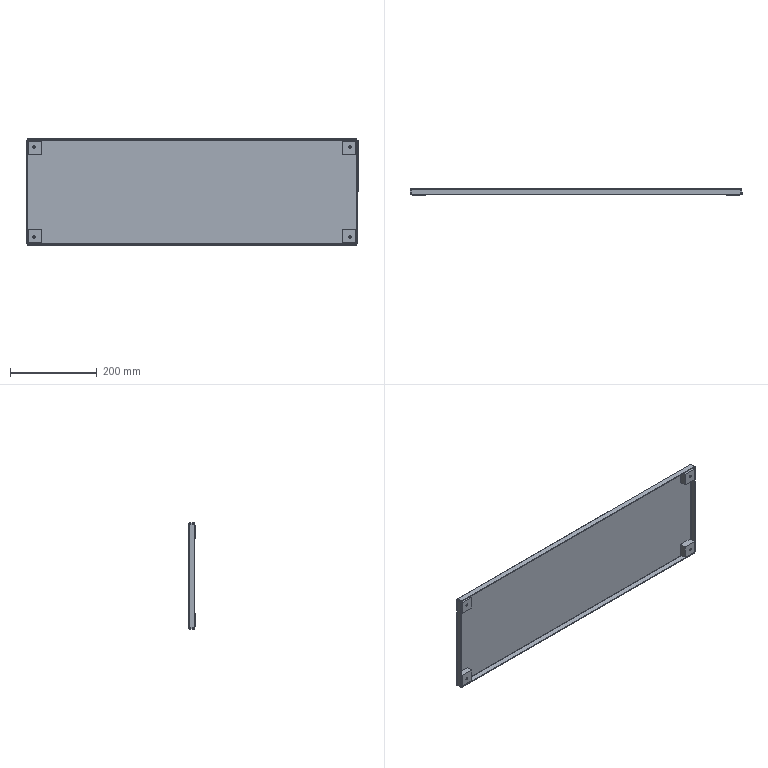Part | SolidWorks | features EdgeFlange 1, FlatPattern 1, HoleWzd 1, ICE 1, SMBaseFlange 1, SheetMetal 1 | 1 solid | 78 faces | box 764 x 16 x 244.5 mm | volume 466147 mm3 | plane 46 | cylinder 24 | spline 8 | commonest cylinder face diameters 5.5 x8 10 x8 1.473 x4 5.473 x4